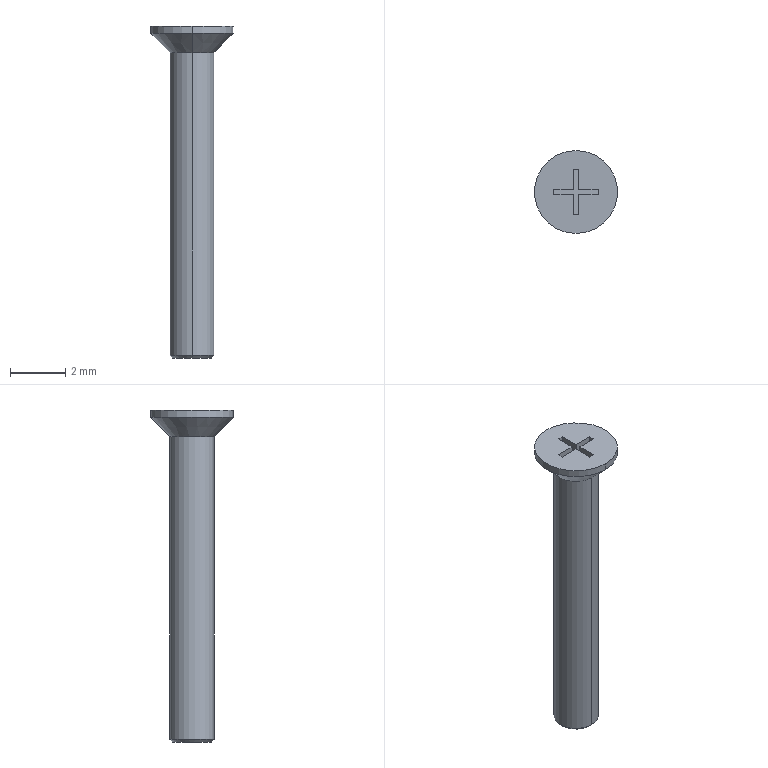Part | STEP file | ASND-0110-0162110302 | 1 solid | 23 faces | box 3 x 3 x 12 mm | volume 26.529 mm3 | plane 15 | cylinder 4 | cone 4 | commonest cylinder face diameters 1.6 x2 3 x2